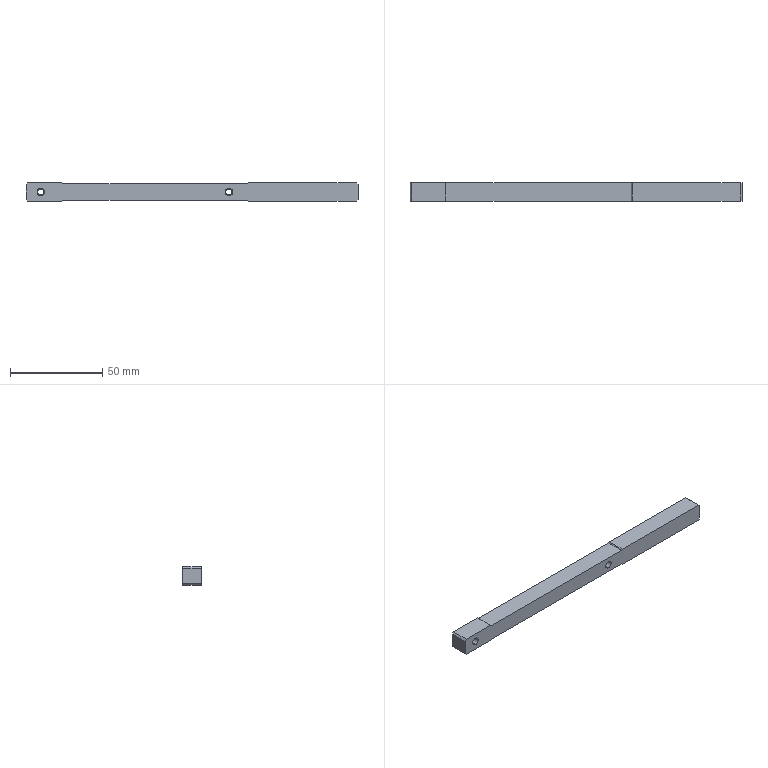Part | SolidWorks | features ICE 4, 3DProfileFeature 2, Chamfer 2, HoleWzd 2, Cut 1, Extrusion 1 | 1 solid | 32 faces | box 180 x 9.8 x 10 mm | volume 15341 mm3 | plane 20 | cylinder 10 | cone 2 | commonest cylinder face diameters 3.3 x4 4.1 x4 5 x2
STEP:
#1=CARTESIAN_POINT('',(110.,5.,1.65));
#2=VERTEX_POINT('',#1);
#3=CARTESIAN_POINT('',(110.,5.,-1.65));
#4=VERTEX_POINT('',#3);
#5=CARTESIAN_POINT('',(110.,5.,0.));
#6=DIRECTION('',(0.,-1.,0.));
#7=DIRECTION('',(0.,0.,-1.));
#8=AXIS2_PLACEMENT_3D('',#5,#6,#7);
#9=CIRCLE('',#8,1.65);
#10=EDGE_CURVE('',#2,#4,#9,.T.);
#11=ORIENTED_EDGE('',*,*,#10,.F.);
#12=CARTESIAN_POINT('',(110.,-0.8,1.65));
#13=VERTEX_POINT('',#12);
#14=CARTESIAN_POINT('',(110.,-0.8,1.65));
#15=DIRECTION('',(0.,-1.,0.));
#16=VECTOR('',#15,1000.);
#17=LINE('',#14,#16);
#18=EDGE_CURVE('',#2,#13,#17,.T.);
#19=ORIENTED_EDGE('',*,*,#18,.T.);
#20=CARTESIAN_POINT('',(110.,-0.8,-1.65));
#21=VERTEX_POINT('',#20);
#22=CARTESIAN_POINT('',(110.,-0.8,0.));
#23=DIRECTION('',(0.,-1.,0.));
#24=DIRECTION('',(0.,0.,-1.));
#25=AXIS2_PLACEMENT_3D('',#22,#23,#24);
#26=CIRCLE('',#25,1.65);
#27=EDGE_CURVE('',#13,#21,#26,.T.);
#28=ORIENTED_EDGE('',*,*,#27,.T.);
#29=CARTESIAN_POINT('',(110.,-0.8,-1.65));
#30=DIRECTION('',(0.,-1.,0.));
#31=VECTOR('',#30,1000.);
#32=LINE('',#29,#31);
#33=EDGE_CURVE('',#4,#21,#32,.T.);
#34=ORIENTED_EDGE('',*,*,#33,.F.);
#35=EDGE_LOOP('',(#11,#19,#28,#34));
#36=FACE_OUTER_BOUND('',#35,.T.);
#37=CARTESIAN_POINT('',(110.,-0.8,0.));
#38=DIRECTION('',(0.,-1.,0.));
#39=DIRECTION('',(0.,0.,-1.));
#40=AXIS2_PLACEMENT_3D('',#37,#38,#39);
#41=CYLINDRICAL_SURFACE('',#40,1.65);
#42=ADVANCED_FACE('',(#36),#41,.F.);
#43=CARTESIAN_POINT('',(8.,5.,1.65));
#44=VERTEX_POINT('',#43);
#45=CARTESIAN_POINT('',(8.,5.,-1.65));
#46=VERTEX_POINT('',#45);
#47=CARTESIAN_POINT('',(8.,5.,0.));
#48=DIRECTION('',(0.,-1.,0.));
#49=DIRECTION('',(0.,0.,-1.));
#50=AXIS2_PLACEMENT_3D('',#47,#48,#49);
#51=CIRCLE('',#50,1.65);
#52=EDGE_CURVE('',#44,#46,#51,.T.);
#53=ORIENTED_EDGE('',*,*,#52,.F.);
#54=CARTESIAN_POINT('',(8.,-0.8,1.65));
#55=VERTEX_POINT('',#54);
#56=CARTESIAN_POINT('',(8.,-0.8,1.65));
#57=DIRECTION('',(0.,-1.,0.));
#58=VECTOR('',#57,1000.);
#59=LINE('',#56,#58);
#60=EDGE_CURVE('',#44,#55,#59,.T.);
#61=ORIENTED_EDGE('',*,*,#60,.T.);
#62=CARTESIAN_POINT('',(8.,-0.8,-1.65));
#63=VERTEX_POINT('',#62);
#64=CARTESIAN_POINT('',(8.,-0.8,0.));
#65=DIRECTION('',(0.,-1.,0.));
#66=DIRECTION('',(0.,0.,-1.));
#67=AXIS2_PLACEMENT_3D('',#64,#65,#66);
#68=CIRCLE('',#67,1.65);
#69=EDGE_CURVE('',#55,#63,#68,.T.);
#70=ORIENTED_EDGE('',*,*,#69,.T.);
#71=CARTESIAN_POINT('',(8.,-0.8,-1.65));
#72=DIRECTION('',(0.,-1.,0.));
#73=VECTOR('',#72,1000.);
#74=LINE('',#71,#73);
#75=EDGE_CURVE('',#46,#63,#74,.T.);
#76=ORIENTED_EDGE('',*,*,#75,.F.);
#77=EDGE_LOOP('',(#53,#61,#70,#76));
#78=FACE_OUTER_BOUND('',#77,.T.);
#79=CARTESIAN_POINT('',(8.,-0.8,0.));
#80=DIRECTION('',(0.,-1.,0.));
#81=DIRECTION('',(0.,0.,-1.));
#82=AXIS2_PLACEMENT_3D('',#79,#80,#81);
#83=CYLINDRICAL_SURFACE('',#82,1.65);
#84=ADVANCED_FACE('',(#78),#83,.F.);
#85=CARTESIAN_POINT('',(110.,-0.8,2.05));
#86=VERTEX_POINT('',#85);
#87=CARTESIAN_POINT('',(110.,-0.8,-2.05));
#88=VERTEX_POINT('',#87);
#89=CARTESIAN_POINT('',(110.,-0.8,0.));
#90=DIRECTION('',(0.,-1.,0.));
#91=DIRECTION('',(0.,0.,-1.));
#92=AXIS2_PLACEMENT_3D('',#89,#90,#91);
#93=CIRCLE('',#92,2.05);
#94=EDGE_CURVE('',#86,#88,#93,.T.);
#95=ORIENTED_EDGE('',*,*,#94,.F.);
#96=CARTESIAN_POINT('',(110.,-4.8,2.05));
#97=VERTEX_POINT('',#96);
#98=CARTESIAN_POINT('',(110.,-0.8,2.05));
#99=DIRECTION('',(0.,-1.,0.));
#100=VECTOR('',#99,1000.);
#101=LINE('',#98,#100);
#102=EDGE_CURVE('',#86,#97,#101,.T.);
#103=ORIENTED_EDGE('',*,*,#102,.T.);
#104=CARTESIAN_POINT('',(110.,-4.8,-2.05));
#105=VERTEX_POINT('',#104);
#106=CARTESIAN_POINT('',(110.,-4.8,0.));
#107=DIRECTION('',(0.,-1.,0.));
#108=DIRECTION('',(0.,0.,-1.));
#109=AXIS2_PLACEMENT_3D('',#106,#107,#108);
#110=CIRCLE('',#109,2.05);
#111=EDGE_CURVE('',#97,#105,#110,.T.);
#112=ORIENTED_EDGE('',*,*,#111,.T.);
#113=CARTESIAN_POINT('',(110.,-0.8,-2.05));
#114=DIRECTION('',(0.,-1.,0.));
#115=VECTOR('',#114,1000.);
#116=LINE('',#113,#115);
#117=EDGE_CURVE('',#88,#105,#116,.T.);
#118=ORIENTED_EDGE('',*,*,#117,.F.);
#119=EDGE_LOOP('',(#95,#103,#112,#118));
#120=FACE_OUTER_BOUND('',#119,.T.);
#121=CARTESIAN_POINT('',(110.,-0.8,0.));
#122=DIRECTION('',(0.,-1.,0.));
#123=DIRECTION('',(0.,0.,-1.));
#124=AXIS2_PLACEMENT_3D('',#121,#122,#123);
#125=CYLINDRICAL_SURFACE('',#124,2.05);
#126=ADVANCED_FACE('',(#120),#125,.F.);
#127=CARTESIAN_POINT('',(8.,-0.8,2.05));
#128=VERTEX_POINT('',#127);
#129=CARTESIAN_POINT('',(8.,-0.8,-2.05));
#130=VERTEX_POINT('',#129);
#131=CARTESIAN_POINT('',(8.,-0.8,0.));
#132=DIRECTION('',(0.,-1.,0.));
#133=DIRECTION('',(0.,0.,-1.));
#134=AXIS2_PLACEMENT_3D('',#131,#132,#133);
#135=CIRCLE('',#134,2.05);
#136=EDGE_CURVE('',#128,#130,#135,.T.);
#137=ORIENTED_EDGE('',*,*,#136,.F.);
#138=CARTESIAN_POINT('',(8.,-4.8,2.05));
#139=VERTEX_POINT('',#138);
#140=CARTESIAN_POINT('',(8.,-0.8,2.05));
#141=DIRECTION('',(0.,-1.,0.));
#142=VECTOR('',#141,1000.);
#143=LINE('',#140,#142);
#144=EDGE_CURVE('',#128,#139,#143,.T.);
#145=ORIENTED_EDGE('',*,*,#144,.T.);
#146=CARTESIAN_POINT('',(8.,-4.8,-2.05));
#147=VERTEX_POINT('',#146);
#148=CARTESIAN_POINT('',(8.,-4.8,0.));
#149=DIRECTION('',(0.,-1.,0.));
#150=DIRECTION('',(0.,0.,-1.));
#151=AXIS2_PLACEMENT_3D('',#148,#149,#150);
#152=CIRCLE('',#151,2.05);
#153=EDGE_CURVE('',#139,#147,#152,.T.);
#154=ORIENTED_EDGE('',*,*,#153,.T.);
#155=CARTESIAN_POINT('',(8.,-0.8,-2.05));
#156=DIRECTION('',(0.,-1.,0.));
#157=VECTOR('',#156,1000.);
#158=LINE('',#155,#157);
#159=EDGE_CURVE('',#130,#147,#158,.T.);
#160=ORIENTED_EDGE('',*,*,#159,.F.);
#161=EDGE_LOOP('',(#137,#145,#154,#160));
#162=FACE_OUTER_BOUND('',#161,.T.);
#163=CARTESIAN_POINT('',(8.,-0.8,0.));
#164=DIRECTION('',(0.,-1.,0.));
#165=DIRECTION('',(0.,0.,-1.));
#166=AXIS2_PLACEMENT_3D('',#163,#164,#165);
#167=CYLINDRICAL_SURFACE('',#166,2.05);
#168=ADVANCED_FACE('',(#162),#167,.F.);
#169=CARTESIAN_POINT('',(125.,0.,2.5));
#170=VERTEX_POINT('',#169);
#171=CARTESIAN_POINT('',(125.,0.,-2.5));
#172=VERTEX_POINT('',#171);
#173=CARTESIAN_POINT('',(125.,0.,0.));
#174=DIRECTION('',(1.,0.,0.));
#175=DIRECTION('',(0.,0.,-1.));
#176=AXIS2_PLACEMENT_3D('',#173,#174,#175);
#177=CIRCLE('',#176,2.5);
#178=EDGE_CURVE('',#170,#172,#177,.T.);
#179=ORIENTED_EDGE('',*,*,#178,.F.);
#180=CARTESIAN_POINT('',(180.,0.,2.5));
#181=VERTEX_POINT('',#180);
#182=CARTESIAN_POINT('',(180.,0.,2.5));
#183=DIRECTION('',(1.,0.,0.));
#184=VECTOR('',#183,1000.);
#185=LINE('',#182,#184);
#186=EDGE_CURVE('',#170,#181,#185,.T.);
#187=ORIENTED_EDGE('',*,*,#186,.T.);
#188=CARTESIAN_POINT('',(180.,0.,-2.5));
#189=VERTEX_POINT('',#188);
#190=CARTESIAN_POINT('',(180.,0.,0.));
#191=DIRECTION('',(1.,0.,0.));
#192=DIRECTION('',(0.,0.,-1.));
#193=AXIS2_PLACEMENT_3D('',#190,#191,#192);
#194=CIRCLE('',#193,2.5);
#195=EDGE_CURVE('',#181,#189,#194,.T.);
#196=ORIENTED_EDGE('',*,*,#195,.T.);
#197=CARTESIAN_POINT('',(180.,0.,-2.5));
#198=DIRECTION('',(1.,0.,0.));
#199=VECTOR('',#198,1000.);
#200=LINE('',#197,#199);
#201=EDGE_CURVE('',#172,#189,#200,.T.);
#202=ORIENTED_EDGE('',*,*,#201,.F.);
#203=EDGE_LOOP('',(#179,#187,#196,#202));
#204=FACE_OUTER_BOUND('',#203,.T.);
#205=CARTESIAN_POINT('',(180.,0.,0.));
#206=DIRECTION('',(1.,0.,0.));
#207=DIRECTION('',(0.,0.,-1.));
#208=AXIS2_PLACEMENT_3D('',#205,#206,#207);
#209=CYLINDRICAL_SURFACE('',#208,2.5);
#210=ADVANCED_FACE('',(#204),#209,.F.);
#211=CARTESIAN_POINT('',(123.498,0.,0.));
#212=VERTEX_POINT('',#211);
#213=CARTESIAN_POINT('',(125.,0.,-2.5));
#214=DIRECTION('',(0.515,0.,-0.8572));
#215=VECTOR('',#214,1000.);
#216=LINE('',#213,#215);
#217=EDGE_CURVE('',#212,#172,#216,.T.);
#218=ORIENTED_EDGE('',*,*,#217,.F.);
#219=CARTESIAN_POINT('',(125.,0.,2.5));
#220=DIRECTION('',(0.515,0.,0.8572));
#221=VECTOR('',#220,1000.);
#222=LINE('',#219,#221);
#223=EDGE_CURVE('',#212,#170,#222,.T.);
#224=ORIENTED_EDGE('',*,*,#223,.T.);
#225=ORIENTED_EDGE('',*,*,#178,.T.);
#226=EDGE_LOOP('',(#218,#224,#225));
#227=FACE_OUTER_BOUND('',#226,.T.);
#228=CARTESIAN_POINT('',(125.,0.,0.));
#229=DIRECTION('',(1.,0.,0.));
#230=DIRECTION('',(0.,0.,-1.));
#231=AXIS2_PLACEMENT_3D('',#228,#229,#230);
#232=CONICAL_SURFACE('',#231,2.5,1.03);
#233=ADVANCED_FACE('',(#227),#232,.F.);
#234=CARTESIAN_POINT('',(179.,5.,-5.));
#235=VERTEX_POINT('',#234);
#236=CARTESIAN_POINT('',(179.,-4.8,-5.));
#237=VERTEX_POINT('',#236);
#238=CARTESIAN_POINT('',(179.,-5.,-5.));
#239=DIRECTION('',(0.,-1.,0.));
#240=VECTOR('',#239,1000.);
#241=LINE('',#238,#240);
#242=EDGE_CURVE('',#235,#237,#241,.T.);
#243=ORIENTED_EDGE('',*,*,#242,.T.);
#244=CARTESIAN_POINT('',(120.5,-4.8,-5.));
#245=VERTEX_POINT('',#244);
#246=CARTESIAN_POINT('',(-180.,-4.8,-5.));
#247=DIRECTION('',(1.,0.,0.));
#248=VECTOR('',#247,1000.);
#249=LINE('',#246,#248);
#250=EDGE_CURVE('',#245,#237,#249,.T.);
#251=ORIENTED_EDGE('',*,*,#250,.F.);
#252=CARTESIAN_POINT('',(120.5,5.,-5.));
#253=VERTEX_POINT('',#252);
#254=CARTESIAN_POINT('',(120.5,5.,-5.));
#255=DIRECTION('',(0.,1.,0.));
#256=VECTOR('',#255,1000.);
#257=LINE('',#254,#256);
#258=EDGE_CURVE('',#245,#253,#257,.T.);
#259=ORIENTED_EDGE('',*,*,#258,.T.);
#260=CARTESIAN_POINT('',(180.,5.,-5.));
#261=DIRECTION('',(-1.,0.,0.));
#262=VECTOR('',#261,1000.);
#263=LINE('',#260,#262);
#264=EDGE_CURVE('',#235,#253,#263,.T.);
#265=ORIENTED_EDGE('',*,*,#264,.F.);
#266=EDGE_LOOP('',(#243,#251,#259,#265));
#267=FACE_OUTER_BOUND('',#266,.T.);
#268=CARTESIAN_POINT('',(180.,5.,-5.));
#269=DIRECTION('',(0.,0.,1.));
#270=DIRECTION('',(0.,-1.,0.));
#271=AXIS2_PLACEMENT_3D('',#268,#269,#270);
#272=PLANE('',#271);
#273=ADVANCED_FACE('',(#267),#272,.F.);
#274=CARTESIAN_POINT('',(1.,5.,5.));
#275=VERTEX_POINT('',#274);
#276=CARTESIAN_POINT('',(1.,-4.8,5.));
#277=VERTEX_POINT('',#276);
#278=CARTESIAN_POINT('',(1.,5.,5.));
#279=DIRECTION('',(0.,-1.,0.));
#280=VECTOR('',#279,1000.);
#281=LINE('',#278,#280);
#282=EDGE_CURVE('',#275,#277,#281,.T.);
#283=ORIENTED_EDGE('',*,*,#282,.T.);
#284=CARTESIAN_POINT('',(19.5,-4.8,5.));
#285=VERTEX_POINT('',#284);
#286=CARTESIAN_POINT('',(-180.,-4.8,5.));
#287=DIRECTION('',(-1.,0.,0.));
#288=VECTOR('',#287,1000.);
#289=LINE('',#286,#288);
#290=EDGE_CURVE('',#285,#277,#289,.T.);
#291=ORIENTED_EDGE('',*,*,#290,.F.);
#292=CARTESIAN_POINT('',(19.5,5.,5.));
#293=VERTEX_POINT('',#292);
#294=CARTESIAN_POINT('',(19.5,5.,5.));
#295=DIRECTION('',(0.,1.,0.));
#296=VECTOR('',#295,1000.);
#297=LINE('',#294,#296);
#298=EDGE_CURVE('',#285,#293,#297,.T.);
#299=ORIENTED_EDGE('',*,*,#298,.T.);
#300=CARTESIAN_POINT('',(180.,5.,5.));
#301=DIRECTION('',(-1.,0.,0.));
#302=VECTOR('',#301,1000.);
#303=LINE('',#300,#302);
#304=EDGE_CURVE('',#293,#275,#303,.T.);
#305=ORIENTED_EDGE('',*,*,#304,.T.);
#306=EDGE_LOOP('',(#283,#291,#299,#305));
#307=FACE_OUTER_BOUND('',#306,.T.);
#308=CARTESIAN_POINT('',(180.,5.,5.));
#309=DIRECTION('',(0.,0.,-1.));
#310=DIRECTION('',(0.,1.,0.));
#311=AXIS2_PLACEMENT_3D('',#308,#309,#310);
#312=PLANE('',#311);
#313=ADVANCED_FACE('',(#307),#312,.F.);
#314=CARTESIAN_POINT('',(19.5,5.,-5.));
#315=VERTEX_POINT('',#314);
#316=CARTESIAN_POINT('',(19.5,-4.8,-5.));
#317=VERTEX_POINT('',#316);
#318=CARTESIAN_POINT('',(19.5,5.,-5.));
#319=DIRECTION('',(0.,-1.,0.));
#320=VECTOR('',#319,1000.);
#321=LINE('',#318,#320);
#322=EDGE_CURVE('',#315,#317,#321,.T.);
#323=ORIENTED_EDGE('',*,*,#322,.T.);
#324=CARTESIAN_POINT('',(1.,-4.8,-5.));
#325=VERTEX_POINT('',#324);
#326=CARTESIAN_POINT('',(-180.,-4.8,-5.));
#327=DIRECTION('',(1.,0.,0.));
#328=VECTOR('',#327,1000.);
#329=LINE('',#326,#328);
#330=EDGE_CURVE('',#325,#317,#329,.T.);
#331=ORIENTED_EDGE('',*,*,#330,.F.);
#332=CARTESIAN_POINT('',(1.,5.,-5.));
#333=VERTEX_POINT('',#332);
#334=CARTESIAN_POINT('',(1.,5.,-5.));
#335=DIRECTION('',(0.,1.,0.));
#336=VECTOR('',#335,1000.);
#337=LINE('',#334,#336);
#338=EDGE_CURVE('',#325,#333,#337,.T.);
#339=ORIENTED_EDGE('',*,*,#338,.T.);
#340=CARTESIAN_POINT('',(180.,5.,-5.));
#341=DIRECTION('',(-1.,0.,0.));
#342=VECTOR('',#341,1000.);
#343=LINE('',#340,#342);
#344=EDGE_CURVE('',#315,#333,#343,.T.);
#345=ORIENTED_EDGE('',*,*,#344,.F.);
#346=EDGE_LOOP('',(#323,#331,#339,#345));
#347=FACE_OUTER_BOUND('',#346,.T.);
#348=CARTESIAN_POINT('',(180.,5.,-5.));
#349=DIRECTION('',(0.,0.,1.));
#350=DIRECTION('',(0.,-1.,0.));
#351=AXIS2_PLACEMENT_3D('',#348,#349,#350);
#352=PLANE('',#351);
#353=ADVANCED_FACE('',(#347),#352,.F.);
#354=CARTESIAN_POINT('',(110.,5.,0.));
#355=DIRECTION('',(0.,-1.,0.));
#356=DIRECTION('',(0.,0.,-1.));
#357=AXIS2_PLACEMENT_3D('',#354,#355,#356);
#358=CIRCLE('',#357,1.65);
#359=EDGE_CURVE('',#4,#2,#358,.T.);
#360=ORIENTED_EDGE('',*,*,#359,.T.);
#361=ORIENTED_EDGE('',*,*,#10,.T.);
#362=EDGE_LOOP('',(#360,#361));
#363=FACE_BOUND('',#362,.T.);
#364=CARTESIAN_POINT('',(8.,5.,0.));
#365=DIRECTION('',(0.,-1.,0.));
#366=DIRECTION('',(0.,0.,-1.));
#367=AXIS2_PLACEMENT_3D('',#364,#365,#366);
#368=CIRCLE('',#367,1.65);
#369=EDGE_CURVE('',#46,#44,#368,.T.);
#370=ORIENTED_EDGE('',*,*,#369,.T.);
#371=ORIENTED_EDGE('',*,*,#52,.T.);
#372=EDGE_LOOP('',(#370,#371));
#373=FACE_BOUND('',#372,.T.);
#374=CARTESIAN_POINT('',(179.,5.,5.));
#375=VERTEX_POINT('',#374);
#376=CARTESIAN_POINT('',(120.5,5.,5.));
#377=VERTEX_POINT('',#376);
#378=CARTESIAN_POINT('',(180.,5.,5.));
#379=DIRECTION('',(-1.,0.,0.));
#380=VECTOR('',#379,1000.);
#381=LINE('',#378,#380);
#382=EDGE_CURVE('',#375,#377,#381,.T.);
#383=ORIENTED_EDGE('',*,*,#382,.F.);
#384=CARTESIAN_POINT('',(180.,5.,4.));
#385=VERTEX_POINT('',#384);
#386=CARTESIAN_POINT('',(180.,5.,4.));
#387=DIRECTION('',(0.7071,0.,-0.7071));
#388=VECTOR('',#387,1000.);
#389=LINE('',#386,#388);
#390=EDGE_CURVE('',#375,#385,#389,.T.);
#391=ORIENTED_EDGE('',*,*,#390,.T.);
#392=CARTESIAN_POINT('',(180.,5.,-4.));
#393=VERTEX_POINT('',#392);
#394=CARTESIAN_POINT('',(180.,5.,5.));
#395=DIRECTION('',(0.,0.,1.));
#396=VECTOR('',#395,1000.);
#397=LINE('',#394,#396);
#398=EDGE_CURVE('',#393,#385,#397,.T.);
#399=ORIENTED_EDGE('',*,*,#398,.F.);
#400=CARTESIAN_POINT('',(180.,5.,-4.));
#401=DIRECTION('',(-0.7071,0.,-0.7071));
#402=VECTOR('',#401,1000.);
#403=LINE('',#400,#402);
#404=EDGE_CURVE('',#393,#235,#403,.T.);
#405=ORIENTED_EDGE('',*,*,#404,.T.);
#406=ORIENTED_EDGE('',*,*,#264,.T.);
#407=CARTESIAN_POINT('',(120.,5.,-4.5));
#408=VERTEX_POINT('',#407);
#409=CARTESIAN_POINT('',(120.5,5.,-5.));
#410=DIRECTION('',(-0.7071,0.,0.7071));
#411=VECTOR('',#410,1000.);
#412=LINE('',#409,#411);
#413=EDGE_CURVE('',#253,#408,#412,.T.);
#414=ORIENTED_EDGE('',*,*,#413,.T.);
#415=CARTESIAN_POINT('',(20.,5.,-4.5));
#416=VERTEX_POINT('',#415);
#417=CARTESIAN_POINT('',(120.,5.,-4.5));
#418=DIRECTION('',(1.,0.,0.));
#419=VECTOR('',#418,1000.);
#420=LINE('',#417,#419);
#421=EDGE_CURVE('',#416,#408,#420,.T.);
#422=ORIENTED_EDGE('',*,*,#421,.F.);
#423=CARTESIAN_POINT('',(19.5,5.,-5.));
#424=DIRECTION('',(-0.7071,0.,-0.7071));
#425=VECTOR('',#424,1000.);
#426=LINE('',#423,#425);
#427=EDGE_CURVE('',#416,#315,#426,.T.);
#428=ORIENTED_EDGE('',*,*,#427,.T.);
#429=ORIENTED_EDGE('',*,*,#344,.T.);
#430=CARTESIAN_POINT('',(0.,5.,-4.));
#431=VERTEX_POINT('',#430);
#432=CARTESIAN_POINT('',(1.,5.,-5.));
#433=DIRECTION('',(-0.7071,0.,0.7071));
#434=VECTOR('',#433,1000.);
#435=LINE('',#432,#434);
#436=EDGE_CURVE('',#333,#431,#435,.T.);
#437=ORIENTED_EDGE('',*,*,#436,.T.);
#438=CARTESIAN_POINT('',(0.,5.,4.));
#439=VERTEX_POINT('',#438);
#440=CARTESIAN_POINT('',(0.,5.,5.));
#441=DIRECTION('',(0.,0.,1.));
#442=VECTOR('',#441,1000.);
#443=LINE('',#440,#442);
#444=EDGE_CURVE('',#431,#439,#443,.T.);
#445=ORIENTED_EDGE('',*,*,#444,.T.);
#446=CARTESIAN_POINT('',(1.,5.,5.));
#447=DIRECTION('',(0.7071,0.,0.7071));
#448=VECTOR('',#447,1000.);
#449=LINE('',#446,#448);
#450=EDGE_CURVE('',#439,#275,#449,.T.);
#451=ORIENTED_EDGE('',*,*,#450,.T.);
#452=ORIENTED_EDGE('',*,*,#304,.F.);
#453=CARTESIAN_POINT('',(20.,5.,4.5));
#454=VERTEX_POINT('',#453);
#455=CARTESIAN_POINT('',(19.5,5.,5.));
#456=DIRECTION('',(0.7071,0.,-0.7071));
#457=VECTOR('',#456,1000.);
#458=LINE('',#455,#457);
#459=EDGE_CURVE('',#293,#454,#458,.T.);
#460=ORIENTED_EDGE('',*,*,#459,.T.);
#461=CARTESIAN_POINT('',(120.,5.,4.5));
#462=VERTEX_POINT('',#461);
#463=CARTESIAN_POINT('',(120.,5.,4.5));
#464=DIRECTION('',(-1.,0.,0.));
#465=VECTOR('',#464,1000.);
#466=LINE('',#463,#465);
#467=EDGE_CURVE('',#462,#454,#466,.T.);
#468=ORIENTED_EDGE('',*,*,#467,.F.);
#469=CARTESIAN_POINT('',(120.5,5.,5.));
#470=DIRECTION('',(0.7071,0.,0.7071));
#471=VECTOR('',#470,1000.);
#472=LINE('',#469,#471);
#473=EDGE_CURVE('',#462,#377,#472,.T.);
#474=ORIENTED_EDGE('',*,*,#473,.T.);
#475=EDGE_LOOP('',(#383,#391,#399,#405,#406,#414,#422,#428,#429,#437,#445,#451,#452,#460,#468,#474));
#476=FACE_OUTER_BOUND('',#475,.T.);
#477=CARTESIAN_POINT('',(180.,5.,5.));
#478=DIRECTION('',(0.,-1.,0.));
#479=DIRECTION('',(0.,0.,-1.));
#480=AXIS2_PLACEMENT_3D('',#477,#478,#479);
#481=PLANE('',#480);
#482=ADVANCED_FACE('',(#363,#373,#476),#481,.F.);
#483=CARTESIAN_POINT('',(120.5,-4.8,5.));
#484=VERTEX_POINT('',#483);
#485=CARTESIAN_POINT('',(120.5,5.,5.));
#486=DIRECTION('',(0.,-1.,0.));
#487=VECTOR('',#486,1000.);
#488=LINE('',#485,#487);
#489=EDGE_CURVE('',#377,#484,#488,.T.);
#490=ORIENTED_EDGE('',*,*,#489,.T.);
#491=CARTESIAN_POINT('',(179.,-4.8,5.));
#492=VERTEX_POINT('',#491);
#493=CARTESIAN_POINT('',(-180.,-4.8,5.));
#494=DIRECTION('',(-1.,0.,0.));
#495=VECTOR('',#494,1000.);
#496=LINE('',#493,#495);
#497=EDGE_CURVE('',#492,#484,#496,.T.);
#498=ORIENTED_EDGE('',*,*,#497,.F.);
#499=CARTESIAN_POINT('',(179.,5.,5.));
#500=DIRECTION('',(0.,1.,0.));
#501=VECTOR('',#500,1000.);
#502=LINE('',#499,#501);
#503=EDGE_CURVE('',#492,#375,#502,.T.);
#504=ORIENTED_EDGE('',*,*,#503,.T.);
#505=ORIENTED_EDGE('',*,*,#382,.T.);
#506=EDGE_LOOP('',(#490,#498,#504,#505));
#507=FACE_OUTER_BOUND('',#506,.T.);
#508=CARTESIAN_POINT('',(180.,5.,5.));
#509=DIRECTION('',(0.,0.,-1.));
#510=DIRECTION('',(0.,1.,0.));
#511=AXIS2_PLACEMENT_3D('',#508,#509,#510);
#512=PLANE('',#511);
#513=ADVANCED_FACE('',(#507),#512,.F.);
#514=CARTESIAN_POINT('',(180.,-4.8,-4.));
#515=VERTEX_POINT('',#514);
#516=CARTESIAN_POINT('',(180.,-4.8,4.));
#517=VERTEX_POINT('',#516);
#518=CARTESIAN_POINT('',(180.,-4.8,-5.));
#519=DIRECTION('',(0.,0.,1.));
#520=VECTOR('',#519,1000.);
#521=LINE('',#518,#520);
#522=EDGE_CURVE('',#515,#517,#521,.T.);
#523=ORIENTED_EDGE('',*,*,#522,.F.);
#524=CARTESIAN_POINT('',(180.,5.,-4.));
#525=DIRECTION('',(0.,1.,0.));
#526=VECTOR('',#525,1000.);
#527=LINE('',#524,#526);
#528=EDGE_CURVE('',#515,#393,#527,.T.);
#529=ORIENTED_EDGE('',*,*,#528,.T.);
#530=ORIENTED_EDGE('',*,*,#398,.T.);
#531=CARTESIAN_POINT('',(180.,-5.,4.));
#532=DIRECTION('',(0.,-1.,0.));
#533=VECTOR('',#532,1000.);
#534=LINE('',#531,#533);
#535=EDGE_CURVE('',#385,#517,#534,.T.);
#536=ORIENTED_EDGE('',*,*,#535,.T.);
#537=EDGE_LOOP('',(#523,#529,#530,#536));
#538=FACE_OUTER_BOUND('',#537,.T.);
#539=CARTESIAN_POINT('',(180.,0.,0.));
#540=DIRECTION('',(1.,0.,0.));
#541=DIRECTION('',(0.,0.,-1.));
#542=AXIS2_PLACEMENT_3D('',#539,#540,#541);
#543=CIRCLE('',#542,2.5);
#544=EDGE_CURVE('',#189,#181,#543,.T.);
#545=ORIENTED_EDGE('',*,*,#544,.F.);
#546=ORIENTED_EDGE('',*,*,#195,.F.);
#547=EDGE_LOOP('',(#545,#546));
#548=FACE_BOUND('',#547,.T.);
#549=CARTESIAN_POINT('',(180.,0.,0.));
#550=DIRECTION('',(1.,0.,0.));
#551=DIRECTION('',(0.,0.,-1.));
#552=AXIS2_PLACEMENT_3D('',#549,#550,#551);
#553=PLANE('',#552);
#554=ADVANCED_FACE('',(#538,#548),#553,.T.);
#555=CARTESIAN_POINT('',(0.,-4.8,-4.));
#556=VERTEX_POINT('',#555);
#557=CARTESIAN_POINT('',(0.,0.,-4.));
#558=DIRECTION('',(0.,-1.,0.));
#559=VECTOR('',#558,1000.);
#560=LINE('',#557,#559);
#561=EDGE_CURVE('',#431,#556,#560,.T.);
#562=ORIENTED_EDGE('',*,*,#561,.T.);
#563=CARTESIAN_POINT('',(0.,-4.8,4.));
#564=VERTEX_POINT('',#563);
#565=CARTESIAN_POINT('',(0.,-4.8,0.));
#566=DIRECTION('',(0.,0.,1.));
#567=VECTOR('',#566,1000.);
#568=LINE('',#565,#567);
#569=EDGE_CURVE('',#556,#564,#568,.T.);
#570=ORIENTED_EDGE('',*,*,#569,.T.);
#571=CARTESIAN_POINT('',(0.,0.,4.));
#572=DIRECTION('',(0.,1.,0.));
#573=VECTOR('',#572,1000.);
#574=LINE('',#571,#573);
#575=EDGE_CURVE('',#564,#439,#574,.T.);
#576=ORIENTED_EDGE('',*,*,#575,.T.);
#577=ORIENTED_EDGE('',*,*,#444,.F.);
#578=EDGE_LOOP('',(#562,#570,#576,#577));
#579=FACE_OUTER_BOUND('',#578,.T.);
#580=CARTESIAN_POINT('',(0.,0.,0.));
#581=DIRECTION('',(1.,0.,0.));
#582=DIRECTION('',(0.,0.,-1.));
#583=AXIS2_PLACEMENT_3D('',#580,#581,#582);
#584=PLANE('',#583);
#585=ADVANCED_FACE('',(#579),#584,.F.);
#586=ORIENTED_EDGE('',*,*,#223,.F.);
#587=ORIENTED_EDGE('',*,*,#217,.T.);
#588=CARTESIAN_POINT('',(125.,0.,0.));
#589=DIRECTION('',(1.,0.,0.));
#590=DIRECTION('',(0.,0.,-1.));
#591=AXIS2_PLACEMENT_3D('',#588,#589,#590);
#592=CIRCLE('',#591,2.5);
#593=EDGE_CURVE('',#172,#170,#592,.T.);
#594=ORIENTED_EDGE('',*,*,#593,.T.);
#595=EDGE_LOOP('',(#586,#587,#594));
#596=FACE_OUTER_BOUND('',#595,.T.);
#597=CARTESIAN_POINT('',(125.,0.,0.));
#598=DIRECTION('',(1.,0.,0.));
#599=DIRECTION('',(0.,0.,-1.));
#600=AXIS2_PLACEMENT_3D('',#597,#598,#599);
#601=CONICAL_SURFACE('',#600,2.5,1.03);
#602=ADVANCED_FACE('',(#596),#601,.F.);
#603=ORIENTED_EDGE('',*,*,#186,.F.);
#604=ORIENTED_EDGE('',*,*,#593,.F.);
#605=ORIENTED_EDGE('',*,*,#201,.T.);
#606=ORIENTED_EDGE('',*,*,#544,.T.);
#607=EDGE_LOOP('',(#603,#604,#605,#606));
#608=FACE_OUTER_BOUND('',#607,.T.);
#609=CARTESIAN_POINT('',(180.,0.,0.));
#610=DIRECTION('',(1.,0.,0.));
#611=DIRECTION('',(0.,0.,-1.));
#612=AXIS2_PLACEMENT_3D('',#609,#610,#611);
#613=CYLINDRICAL_SURFACE('',#612,2.5);
#614=ADVANCED_FACE('',(#608),#613,.F.);
#615=CARTESIAN_POINT('',(20.,-4.8,4.5));
#616=VERTEX_POINT('',#615);
#617=CARTESIAN_POINT('',(20.,-5.,4.5));
#618=DIRECTION('',(0.,1.,0.));
#619=VECTOR('',#618,1000.);
#620=LINE('',#617,#619);
#621=EDGE_CURVE('',#616,#454,#620,.T.);
#622=ORIENTED_EDGE('',*,*,#621,.F.);
#623=CARTESIAN_POINT('',(120.,-4.8,4.5));
#624=VERTEX_POINT('',#623);
#625=CARTESIAN_POINT('',(120.,-4.8,4.5));
#626=DIRECTION('',(1.,0.,0.));
#627=VECTOR('',#626,1000.);
#628=LINE('',#625,#627);
#629=EDGE_CURVE('',#616,#624,#628,.T.);
#630=ORIENTED_EDGE('',*,*,#629,.T.);
#631=CARTESIAN_POINT('',(120.,-5.,4.5));
#632=DIRECTION('',(0.,1.,0.));
#633=VECTOR('',#632,1000.);
#634=LINE('',#631,#633);
#635=EDGE_CURVE('',#624,#462,#634,.T.);
#636=ORIENTED_EDGE('',*,*,#635,.T.);
#637=ORIENTED_EDGE('',*,*,#467,.T.);
#638=EDGE_LOOP('',(#622,#630,#636,#637));
#639=FACE_OUTER_BOUND('',#638,.T.);
#640=CARTESIAN_POINT('',(120.,-5.,4.5));
#641=DIRECTION('',(0.,0.,-1.));
#642=DIRECTION('',(-1.,0.,0.));
#643=AXIS2_PLACEMENT_3D('',#640,#641,#642);
#644=PLANE('',#643);
#645=ADVANCED_FACE('',(#639),#644,.F.);
#646=CARTESIAN_POINT('',(120.,-4.8,-4.5));
#647=VERTEX_POINT('',#646);
#648=CARTESIAN_POINT('',(120.,-5.,-4.5));
#649=DIRECTION('',(0.,1.,0.));
#650=VECTOR('',#649,1000.);
#651=LINE('',#648,#650);
#652=EDGE_CURVE('',#647,#408,#651,.T.);
#653=ORIENTED_EDGE('',*,*,#652,.F.);
#654=CARTESIAN_POINT('',(20.,-4.8,-4.5));
#655=VERTEX_POINT('',#654);
#656=CARTESIAN_POINT('',(120.,-4.8,-4.5));
#657=DIRECTION('',(-1.,0.,0.));
#658=VECTOR('',#657,1000.);
#659=LINE('',#656,#658);
#660=EDGE_CURVE('',#647,#655,#659,.T.);
#661=ORIENTED_EDGE('',*,*,#660,.T.);
#662=CARTESIAN_POINT('',(20.,-5.,-4.5));
#663=DIRECTION('',(0.,1.,0.));
#664=VECTOR('',#663,1000.);
#665=LINE('',#662,#664);
#666=EDGE_CURVE('',#655,#416,#665,.T.);
#667=ORIENTED_EDGE('',*,*,#666,.T.);
#668=ORIENTED_EDGE('',*,*,#421,.T.);
#669=EDGE_LOOP('',(#653,#661,#667,#668));
#670=FACE_OUTER_BOUND('',#669,.T.);
#671=CARTESIAN_POINT('',(120.,-5.,-4.5));
#672=DIRECTION('',(0.,0.,1.));
#673=DIRECTION('',(1.,0.,0.));
#674=AXIS2_PLACEMENT_3D('',#671,#672,#673);
#675=PLANE('',#674);
#676=ADVANCED_FACE('',(#670),#675,.F.);
#677=CARTESIAN_POINT('',(19.5,-4.8,-5.));
#678=DIRECTION('',(0.7071,0.,0.7071));
#679=VECTOR('',#678,1000.);
#680=LINE('',#677,#679);
#681=EDGE_CURVE('',#317,#655,#680,.T.);
#682=ORIENTED_EDGE('',*,*,#681,.F.);
#683=ORIENTED_EDGE('',*,*,#322,.F.);
#684=ORIENTED_EDGE('',*,*,#427,.F.);
#685=ORIENTED_EDGE('',*,*,#666,.F.);
#686=EDGE_LOOP('',(#682,#683,#684,#685));
#687=FACE_OUTER_BOUND('',#686,.T.);
#688=CARTESIAN_POINT('',(19.5,5.,-5.));
#689=DIRECTION('',(-0.7071,0.,0.7071));
#690=DIRECTION('',(0.,-1.,0.));
#691=AXIS2_PLACEMENT_3D('',#688,#689,#690);
#692=PLANE('',#691);
#693=ADVANCED_FACE('',(#687),#692,.F.);
#694=CARTESIAN_POINT('',(19.5,-4.8,5.));
#695=DIRECTION('',(-0.7071,0.,0.7071));
#696=VECTOR('',#695,1000.);
#697=LINE('',#694,#696);
#698=EDGE_CURVE('',#616,#285,#697,.T.);
#699=ORIENTED_EDGE('',*,*,#698,.F.);
#700=ORIENTED_EDGE('',*,*,#621,.T.);
#701=ORIENTED_EDGE('',*,*,#459,.F.);
#702=ORIENTED_EDGE('',*,*,#298,.F.);
#703=EDGE_LOOP('',(#699,#700,#701,#702));
#704=FACE_OUTER_BOUND('',#703,.T.);
#705=CARTESIAN_POINT('',(19.5,5.,5.));
#706=DIRECTION('',(-0.7071,0.,-0.7071));
#707=DIRECTION('',(0.,1.,0.));
#708=AXIS2_PLACEMENT_3D('',#705,#706,#707);
#709=PLANE('',#708);
#710=ADVANCED_FACE('',(#704),#709,.F.);
#711=CARTESIAN_POINT('',(120.5,-4.8,5.));
#712=DIRECTION('',(-0.7071,0.,-0.7071));
#713=VECTOR('',#712,1000.);
#714=LINE('',#711,#713);
#715=EDGE_CURVE('',#484,#624,#714,.T.);
#716=ORIENTED_EDGE('',*,*,#715,.F.);
#717=ORIENTED_EDGE('',*,*,#489,.F.);
#718=ORIENTED_EDGE('',*,*,#473,.F.);
#719=ORIENTED_EDGE('',*,*,#635,.F.);
#720=EDGE_LOOP('',(#716,#717,#718,#719));
#721=FACE_OUTER_BOUND('',#720,.T.);
#722=CARTESIAN_POINT('',(120.5,5.,5.));
#723=DIRECTION('',(0.7071,0.,-0.7071));
#724=DIRECTION('',(0.,-1.,0.));
#725=AXIS2_PLACEMENT_3D('',#722,#723,#724);
#726=PLANE('',#725);
#727=ADVANCED_FACE('',(#721),#726,.F.);
#728=CARTESIAN_POINT('',(120.5,-4.8,-5.));
#729=DIRECTION('',(0.7071,0.,-0.7071));
#730=VECTOR('',#729,1000.);
#731=LINE('',#728,#730);
#732=EDGE_CURVE('',#647,#245,#731,.T.);
#733=ORIENTED_EDGE('',*,*,#732,.F.);
#734=ORIENTED_EDGE('',*,*,#652,.T.);
#735=ORIENTED_EDGE('',*,*,#413,.F.);
#736=ORIENTED_EDGE('',*,*,#258,.F.);
#737=EDGE_LOOP('',(#733,#734,#735,#736));
#738=FACE_OUTER_BOUND('',#737,.T.);
#739=CARTESIAN_POINT('',(120.5,5.,-5.));
#740=DIRECTION('',(0.7071,0.,0.7071));
#741=DIRECTION('',(0.,1.,0.));
#742=AXIS2_PLACEMENT_3D('',#739,#740,#741);
#743=PLANE('',#742);
#744=ADVANCED_FACE('',(#738),#743,.F.);
#745=CARTESIAN_POINT('',(180.,-4.8,4.));
#746=DIRECTION('',(-0.7071,0.,0.7071));
#747=VECTOR('',#746,1000.);
#748=LINE('',#745,#747);
#749=EDGE_CURVE('',#517,#492,#748,.T.);
#750=ORIENTED_EDGE('',*,*,#749,.F.);
#751=ORIENTED_EDGE('',*,*,#535,.F.);
#752=ORIENTED_EDGE('',*,*,#390,.F.);
#753=ORIENTED_EDGE('',*,*,#503,.F.);
#754=EDGE_LOOP('',(#750,#751,#752,#753));
#755=FACE_OUTER_BOUND('',#754,.T.);
#756=CARTESIAN_POINT('',(180.,0.,4.));
#757=DIRECTION('',(0.7071,0.,0.7071));
#758=DIRECTION('',(0.,1.,0.));
#759=AXIS2_PLACEMENT_3D('',#756,#757,#758);
#760=PLANE('',#759);
#761=ADVANCED_FACE('',(#755),#760,.T.);
#762=CARTESIAN_POINT('',(180.,-4.8,-4.));
#763=DIRECTION('',(0.7071,0.,0.7071));
#764=VECTOR('',#763,1000.);
#765=LINE('',#762,#764);
#766=EDGE_CURVE('',#237,#515,#765,.T.);
#767=ORIENTED_EDGE('',*,*,#766,.F.);
#768=ORIENTED_EDGE('',*,*,#242,.F.);
#769=ORIENTED_EDGE('',*,*,#404,.F.);
#770=ORIENTED_EDGE('',*,*,#528,.F.);
#771=EDGE_LOOP('',(#767,#768,#769,#770));
#772=FACE_OUTER_BOUND('',#771,.T.);
#773=CARTESIAN_POINT('',(180.,0.,-4.));
#774=DIRECTION('',(0.7071,0.,-0.7071));
#775=DIRECTION('',(0.,-1.,0.));
#776=AXIS2_PLACEMENT_3D('',#773,#774,#775);
#777=PLANE('',#776);
#778=ADVANCED_FACE('',(#772),#777,.T.);
#779=CARTESIAN_POINT('',(1.,-4.8,5.));
#780=DIRECTION('',(-0.7071,0.,-0.7071));
#781=VECTOR('',#780,1000.);
#782=LINE('',#779,#781);
#783=EDGE_CURVE('',#277,#564,#782,.T.);
#784=ORIENTED_EDGE('',*,*,#783,.F.);
#785=ORIENTED_EDGE('',*,*,#282,.F.);
#786=ORIENTED_EDGE('',*,*,#450,.F.);
#787=ORIENTED_EDGE('',*,*,#575,.F.);
#788=EDGE_LOOP('',(#784,#785,#786,#787));
#789=FACE_OUTER_BOUND('',#788,.T.);
#790=CARTESIAN_POINT('',(1.,5.,5.));
#791=DIRECTION('',(0.7071,0.,-0.7071));
#792=DIRECTION('',(0.,-1.,0.));
#793=AXIS2_PLACEMENT_3D('',#790,#791,#792);
#794=PLANE('',#793);
#795=ADVANCED_FACE('',(#789),#794,.F.);
#796=CARTESIAN_POINT('',(1.,-4.8,-5.));
#797=DIRECTION('',(0.7071,0.,-0.7071));
#798=VECTOR('',#797,1000.);
#799=LINE('',#796,#798);
#800=EDGE_CURVE('',#556,#325,#799,.T.);
#801=ORIENTED_EDGE('',*,*,#800,.F.);
#802=ORIENTED_EDGE('',*,*,#561,.F.);
#803=ORIENTED_EDGE('',*,*,#436,.F.);
#804=ORIENTED_EDGE('',*,*,#338,.F.);
#805=EDGE_LOOP('',(#801,#802,#803,#804));
#806=FACE_OUTER_BOUND('',#805,.T.);
#807=CARTESIAN_POINT('',(1.,5.,-5.));
#808=DIRECTION('',(0.7071,0.,0.7071));
#809=DIRECTION('',(0.,1.,0.));
#810=AXIS2_PLACEMENT_3D('',#807,#808,#809);
#811=PLANE('',#810);
#812=ADVANCED_FACE('',(#806),#811,.F.);
#813=CARTESIAN_POINT('',(110.,-4.8,0.));
#814=DIRECTION('',(0.,-1.,0.));
#815=DIRECTION('',(0.,0.,-1.));
#816=AXIS2_PLACEMENT_3D('',#813,#814,#815);
#817=CIRCLE('',#816,2.05);
#818=EDGE_CURVE('',#105,#97,#817,.T.);
#819=ORIENTED_EDGE('',*,*,#818,.F.);
#820=ORIENTED_EDGE('',*,*,#111,.F.);
#821=EDGE_LOOP('',(#819,#820));
#822=FACE_BOUND('',#821,.T.);
#823=CARTESIAN_POINT('',(8.,-4.8,0.));
#824=DIRECTION('',(0.,-1.,0.));
#825=DIRECTION('',(0.,0.,-1.));
#826=AXIS2_PLACEMENT_3D('',#823,#824,#825);
#827=CIRCLE('',#826,2.05);
#828=EDGE_CURVE('',#147,#139,#827,.T.);
#829=ORIENTED_EDGE('',*,*,#828,.F.);
#830=ORIENTED_EDGE('',*,*,#153,.F.);
#831=EDGE_LOOP('',(#829,#830));
#832=FACE_BOUND('',#831,.T.);
#833=ORIENTED_EDGE('',*,*,#698,.T.);
#834=ORIENTED_EDGE('',*,*,#290,.T.);
#835=ORIENTED_EDGE('',*,*,#783,.T.);
#836=ORIENTED_EDGE('',*,*,#569,.F.);
#837=ORIENTED_EDGE('',*,*,#800,.T.);
#838=ORIENTED_EDGE('',*,*,#330,.T.);
#839=ORIENTED_EDGE('',*,*,#681,.T.);
#840=ORIENTED_EDGE('',*,*,#660,.F.);
#841=ORIENTED_EDGE('',*,*,#732,.T.);
#842=ORIENTED_EDGE('',*,*,#250,.T.);
#843=ORIENTED_EDGE('',*,*,#766,.T.);
#844=ORIENTED_EDGE('',*,*,#522,.T.);
#845=ORIENTED_EDGE('',*,*,#749,.T.);
#846=ORIENTED_EDGE('',*,*,#497,.T.);
#847=ORIENTED_EDGE('',*,*,#715,.T.);
#848=ORIENTED_EDGE('',*,*,#629,.F.);
#849=EDGE_LOOP('',(#833,#834,#835,#836,#837,#838,#839,#840,#841,#842,#843,#844,#845,#846,#847,#848));
#850=FACE_OUTER_BOUND('',#849,.T.);
#851=CARTESIAN_POINT('',(0.,-4.8,0.));
#852=DIRECTION('',(0.,1.,0.));
#853=DIRECTION('',(0.,0.,1.));
#854=AXIS2_PLACEMENT_3D('',#851,#852,#853);
#855=PLANE('',#854);
#856=ADVANCED_FACE('',(#822,#832,#850),#855,.F.);
#857=CARTESIAN_POINT('',(8.,-0.8,0.));
#858=DIRECTION('',(0.,-1.,0.));
#859=DIRECTION('',(0.,0.,-1.));
#860=AXIS2_PLACEMENT_3D('',#857,#858,#859);
#861=CIRCLE('',#860,1.65);
#862=EDGE_CURVE('',#63,#55,#861,.T.);
#863=ORIENTED_EDGE('',*,*,#862,.F.);
#864=ORIENTED_EDGE('',*,*,#69,.F.);
#865=EDGE_LOOP('',(#863,#864));
#866=FACE_BOUND('',#865,.T.);
#867=CARTESIAN_POINT('',(8.,-0.8,0.));
#868=DIRECTION('',(0.,-1.,0.));
#869=DIRECTION('',(0.,0.,-1.));
#870=AXIS2_PLACEMENT_3D('',#867,#868,#869);
#871=CIRCLE('',#870,2.05);
#872=EDGE_CURVE('',#130,#128,#871,.T.);
#873=ORIENTED_EDGE('',*,*,#872,.T.);
#874=ORIENTED_EDGE('',*,*,#136,.T.);
#875=EDGE_LOOP('',(#873,#874));
#876=FACE_OUTER_BOUND('',#875,.T.);
#877=CARTESIAN_POINT('',(8.,-0.8,0.));
#878=DIRECTION('',(0.,-1.,0.));
#879=DIRECTION('',(0.,0.,-1.));
#880=AXIS2_PLACEMENT_3D('',#877,#878,#879);
#881=PLANE('',#880);
#882=ADVANCED_FACE('',(#866,#876),#881,.T.);
#883=ORIENTED_EDGE('',*,*,#144,.F.);
#884=ORIENTED_EDGE('',*,*,#872,.F.);
#885=ORIENTED_EDGE('',*,*,#159,.T.);
#886=ORIENTED_EDGE('',*,*,#828,.T.);
#887=EDGE_LOOP('',(#883,#884,#885,#886));
#888=FACE_OUTER_BOUND('',#887,.T.);
#889=CARTESIAN_POINT('',(8.,-0.8,0.));
#890=DIRECTION('',(0.,-1.,0.));
#891=DIRECTION('',(0.,0.,-1.));
#892=AXIS2_PLACEMENT_3D('',#889,#890,#891);
#893=CYLINDRICAL_SURFACE('',#892,2.05);
#894=ADVANCED_FACE('',(#888),#893,.F.);
#895=CARTESIAN_POINT('',(110.,-0.8,0.));
#896=DIRECTION('',(0.,-1.,0.));
#897=DIRECTION('',(0.,0.,-1.));
#898=AXIS2_PLACEMENT_3D('',#895,#896,#897);
#899=CIRCLE('',#898,1.65);
#900=EDGE_CURVE('',#21,#13,#899,.T.);
#901=ORIENTED_EDGE('',*,*,#900,.F.);
#902=ORIENTED_EDGE('',*,*,#27,.F.);
#903=EDGE_LOOP('',(#901,#902));
#904=FACE_BOUND('',#903,.T.);
#905=CARTESIAN_POINT('',(110.,-0.8,0.));
#906=DIRECTION('',(0.,-1.,0.));
#907=DIRECTION('',(0.,0.,-1.));
#908=AXIS2_PLACEMENT_3D('',#905,#906,#907);
#909=CIRCLE('',#908,2.05);
#910=EDGE_CURVE('',#88,#86,#909,.T.);
#911=ORIENTED_EDGE('',*,*,#910,.T.);
#912=ORIENTED_EDGE('',*,*,#94,.T.);
#913=EDGE_LOOP('',(#911,#912));
#914=FACE_OUTER_BOUND('',#913,.T.);
#915=CARTESIAN_POINT('',(110.,-0.8,0.));
#916=DIRECTION('',(0.,-1.,0.));
#917=DIRECTION('',(0.,0.,-1.));
#918=AXIS2_PLACEMENT_3D('',#915,#916,#917);
#919=PLANE('',#918);
#920=ADVANCED_FACE('',(#904,#914),#919,.T.);
#921=ORIENTED_EDGE('',*,*,#102,.F.);
#922=ORIENTED_EDGE('',*,*,#910,.F.);
#923=ORIENTED_EDGE('',*,*,#117,.T.);
#924=ORIENTED_EDGE('',*,*,#818,.T.);
#925=EDGE_LOOP('',(#921,#922,#923,#924));
#926=FACE_OUTER_BOUND('',#925,.T.);
#927=CARTESIAN_POINT('',(110.,-0.8,0.));
#928=DIRECTION('',(0.,-1.,0.));
#929=DIRECTION('',(0.,0.,-1.));
#930=AXIS2_PLACEMENT_3D('',#927,#928,#929);
#931=CYLINDRICAL_SURFACE('',#930,2.05);
#932=ADVANCED_FACE('',(#926),#931,.F.);
#933=ORIENTED_EDGE('',*,*,#60,.F.);
#934=ORIENTED_EDGE('',*,*,#369,.F.);
#935=ORIENTED_EDGE('',*,*,#75,.T.);
#936=ORIENTED_EDGE('',*,*,#862,.T.);
#937=EDGE_LOOP('',(#933,#934,#935,#936));
#938=FACE_OUTER_BOUND('',#937,.T.);
#939=CARTESIAN_POINT('',(8.,-0.8,0.));
#940=DIRECTION('',(0.,-1.,0.));
#941=DIRECTION('',(0.,0.,-1.));
#942=AXIS2_PLACEMENT_3D('',#939,#940,#941);
#943=CYLINDRICAL_SURFACE('',#942,1.65);
#944=ADVANCED_FACE('',(#938),#943,.F.);
#945=ORIENTED_EDGE('',*,*,#18,.F.);
#946=ORIENTED_EDGE('',*,*,#359,.F.);
#947=ORIENTED_EDGE('',*,*,#33,.T.);
#948=ORIENTED_EDGE('',*,*,#900,.T.);
#949=EDGE_LOOP('',(#945,#946,#947,#948));
#950=FACE_OUTER_BOUND('',#949,.T.);
#951=CARTESIAN_POINT('',(110.,-0.8,0.));
#952=DIRECTION('',(0.,-1.,0.));
#953=DIRECTION('',(0.,0.,-1.));
#954=AXIS2_PLACEMENT_3D('',#951,#952,#953);
#955=CYLINDRICAL_SURFACE('',#954,1.65);
#956=ADVANCED_FACE('',(#950),#955,.F.);
#957=CLOSED_SHELL('',(#42,#84,#126,#168,#210,#233,#273,#313,#353,#482,#513,#554,#585,#602,#614,#645,#676,#693,#710,#727,#744,#761,#778,#795,#812,#856,#882,#894,#920,#932,#944,#956));
#958=MANIFOLD_SOLID_BREP('',#957);
#959=CARTESIAN_POINT('',(0.,0.,0.));
#960=DIRECTION('',(0.,0.,1.));
#961=DIRECTION('',(1.,0.,0.));
#962=AXIS2_PLACEMENT_3D('',#959,#960,#961);
#963=(LENGTH_UNIT()NAMED_UNIT(*)SI_UNIT(.MILLI.,.METRE.));
#964=UNCERTAINTY_MEASURE_WITH_UNIT(LENGTH_MEASURE(0.00001),#963,'','');
#965=(NAMED_UNIT(*)PLANE_ANGLE_UNIT()SI_UNIT($,.RADIAN.));
#966=(NAMED_UNIT(*)SI_UNIT($,.STERADIAN.)SOLID_ANGLE_UNIT());
#967=(GEOMETRIC_REPRESENTATION_CONTEXT(3)GLOBAL_UNCERTAINTY_ASSIGNED_CONTEXT((#964))GLOBAL_UNIT_ASSIGNED_CONTEXT((#963,#965,#966))REPRESENTATION_CONTEXT('',''));
#968=ADVANCED_BREP_SHAPE_REPRESENTATION('',(#958,#962),#967);